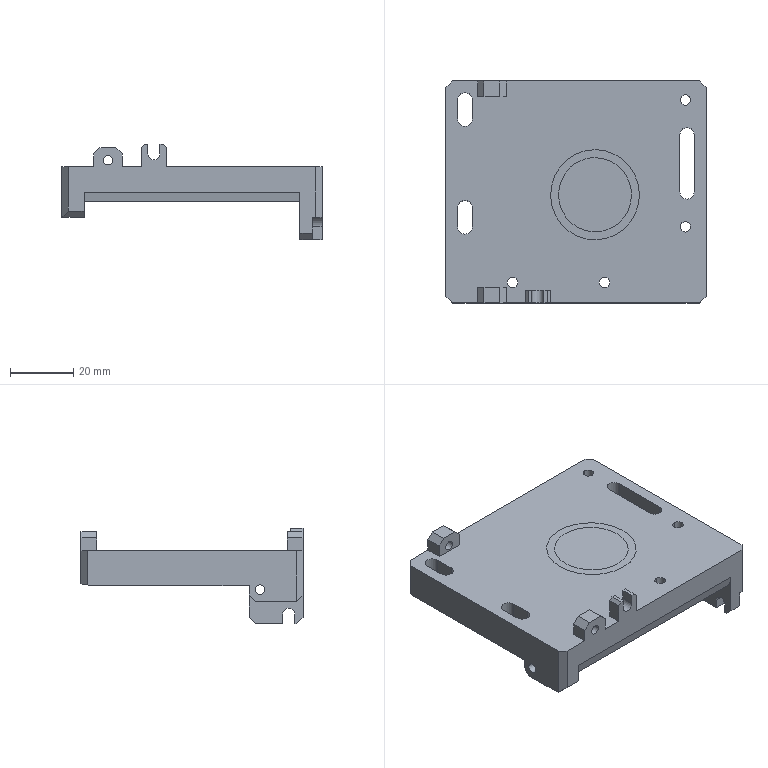NC program | NX | posted with a generic post | part box 82 x 70 x 30 mm
Lines 2139 to 2435 of 2435:
(FIXED_CONTOUR_COPY , TOOL : D3R0.5)
N4240 T05 M6
N4242 G54
N4244 G17 G0 G90 X-35.934 Y-39.23 B0. C0. S9500 M3
N4246 G43 Z30. H5
N4248 Z-9.
N4250 G94 G1 Z-12.53 F1000.
N4252 G2 X-36.039 Y-39.048 R0.21
N4254 G1 Y39.048 F2000.
N4256 X-35.992 Y39.095 Z-12.52
N4258 Y-39.095
N4260 X-35.945 Y-39.142 Z-12.512
N4262 Y39.142
N4264 X-35.897 Y39.189 Z-12.503
N4266 Y-39.189
N4268 X-35.85 Y-39.237 Z-12.495
N4270 Y39.237
N4272 X-35.803 Y39.284 Z-12.487
N4274 Y-39.284
N4276 X-35.756 Y-39.331 Z-12.478
N4278 Y39.331
N4280 X-35.709 Y39.378 Z-12.47
N4282 Y-39.378
N4284 X-35.662 Y-39.425 Z-12.462
N4286 Y39.425
N4288 X-35.614 Y39.472 Z-12.453
N4290 Y-39.472
N4292 X-35.567 Y-39.52 Z-12.445
N4294 Y39.52
N4296 X-35.52 Y39.567 Z-12.437
N4298 Y-39.567
N4300 X-35.473 Y-39.614 Z-12.428
N4302 Y39.614
N4304 X-35.426 Y39.661 Z-12.42
N4306 Y-39.661
N4308 X-35.378 Y-39.709 Z-12.412
N4310 Y39.709
N4312 X-35.331 Y39.756 Z-12.403
N4314 Y-39.756
N4316 X-35.284 Y-39.803 Z-12.395
N4318 Y39.803
N4320 X-35.236 Y39.851 Z-12.387
N4322 Y-39.851
N4324 X-35.189 Y-39.898 Z-12.378
N4326 Y39.898
N4328 X-35.142 Y39.945 Z-12.37
N4330 Y-39.945
N4332 X-35.094 Y-39.993 Z-12.362
N4334 Y39.993
N4336 X-35.047 Y40.04 Z-12.353
N4338 Y-40.04
N4340 X-35. Y-40.087 Z-12.345
N4342 Y40.087
N4344 X-34.952 Y40.135 Z-12.337
N4346 Y-40.135
N4348 X-34.905 Y-40.182 Z-12.328
N4350 Y40.182
N4352 X-34.857 Y40.23 Z-12.32
N4354 Y-40.23
N4356 X-34.81 Y-40.277 Z-12.311
N4358 Y40.277
N4360 X-34.763 Y40.324 Z-12.303
N4362 Y-40.324
N4364 X-34.715 Y-40.372 Z-12.295
N4366 Y40.372
N4368 X-34.668 Y40.419 Z-12.286
N4370 Y-40.419
N4372 X-34.62 Y-40.467 Z-12.278
N4374 Y40.467
N4376 X-34.573 Y40.514 Z-12.27
N4378 Y-40.514
N4380 X-34.526 Y-40.561 Z-12.261
N4382 Y40.561
N4384 X-34.478 Y40.609 Z-12.253
N4386 Y-40.609
N4388 X-34.431 Y-40.656 Z-12.245
N4390 Y40.656
N4392 X-34.383 Y40.703 Z-12.236
N4394 Y-40.703
N4396 X-34.336 Y-40.751 Z-12.228
N4398 Y40.751
N4400 X-34.289 Y40.798 Z-12.22
N4402 Y-40.798
N4404 X-34.242 Y-40.845 Z-12.211
N4406 X-34.241 Y40.845
N4408 X-34.194 Y40.893 Z-12.203
N4410 Y-40.893
N4412 X-34.147 Y-40.94 Z-12.195
N4414 Y40.94
N4416 X-34.099 Y40.988 Z-12.187
N4418 Y38.314 Z-12.186
N4420 Y-40.868
N4422 Y-40.988 Z-12.187
N4424 X-34.087 Y-41. Z-12.185
N4426 X-34.05 Z-12.179
N4428 Y-40.23 Z-12.177
N4430 Y40.868
N4432 Y41. Z-12.179
N4434 X-34.001 Z-12.17
N4436 Y40.23 Z-12.169
N4438 Y-40.868
N4440 Y-41. Z-12.17
N4442 X-33.951 Z-12.161
N4444 Y-40.23 Z-12.16
N4446 Y40.868
N4448 Y41. Z-12.161
N4450 X-33.902 Z-12.153
N4452 Y40.233 Z-12.151
N4454 Y-40.864
N4456 Y-41. Z-12.153
N4458 X-33.853 Z-12.144
N4460 Y-40.23 Z-12.143
N4462 Y40.868
N4464 Y41. Z-12.144
N4466 X-33.804 Z-12.135
N4468 Y40.23 Z-12.134
N4470 Y-40.868
N4472 Y-41. Z-12.135
N4474 X-33.754 Z-12.127
N4476 Y-40.23 Z-12.125
N4478 Y40.868
N4480 Y41. Z-12.127
N4482 X-33.705 Z-12.118
N4484 Y40.23 Z-12.117
N4486 Y-40.868
N4488 Y-41. Z-12.118
N4490 X-33.656 Z-12.109
N4492 Y-40.23 Z-12.108
N4494 Y40.868
N4496 Y41. Z-12.109
N4498 X-33.607 Z-12.101
N4500 Y40.23 Z-12.099
N4502 Y-40.868
N4504 Y-41. Z-12.101
N4506 X-33.557 Z-12.092
N4508 Y-40.23 Z-12.091
N4510 Y40.871
N4512 Y41. Z-12.092
N4514 X-33.508 Z-12.083
N4516 Y40.23 Z-12.082
N4518 Y-40.868
N4520 Y-41. Z-12.083
N4522 X-33.459 Z-12.075
N4524 Y-40.23 Z-12.073
N4526 Y40.868
N4528 Y41. Z-12.075
N4530 X-33.41 Z-12.066
N4532 Y40.23 Z-12.065
N4534 Y-40.868
N4536 Y-41. Z-12.066
N4538 X-33.36 Z-12.057
N4540 Y-40.23 Z-12.056
N4542 Y40.868
N4544 Y41. Z-12.057
N4546 X-33.311 Z-12.049
N4548 Y40.23 Z-12.047
N4550 Y-40.868
N4552 Y-41. Z-12.049
N4554 X-33.262 Z-12.04
N4556 Y-40.23 Z-12.038
N4558 Y40.868
N4560 Y41. Z-12.04
N4562 X-33.213 Z-12.031
N4564 Y40.233 Z-12.03
N4566 Y-40.868
N4568 Y-41. Z-12.031
N4570 X-33.163 Z-12.023
N4572 Y41.
N4574 X-33.114 Z-12.015
N4576 Y-41.
N4578 G2 X-33.264 Y-41.26 R0.3
N4580 G1 Z-9.
N4582 G0 Z30.
(ZLEVEL_PROFILE_1_COPY_COPY , TOOL : D3R0.5)
N4584 X36.666 Y32.722
N4586 Z-10.598
N4588 G1 Z-12.098 F1000.
N4590 X36.21 Y32.873
N4592 G3 X35.916 Y32.812 R0.3
N4594 G1 X35.908 Y32.805 F2500.
N4596 Y-32.805
N4598 X35.916 Y-32.812
N4600 X35.925 Y-32.819 Z-12.197
N4602 Y32.819
N4604 X35.943 Y32.833 Z-12.295
N4606 Y-32.833
N4608 X35.96 Y-32.848 Z-12.394
N4610 Y32.848
N4612 X35.977 Y32.862 Z-12.492
N4614 Y-32.862
N4616 X35.995 Y-32.877 Z-12.591
N4618 Y32.877
N4620 X36.012 Y32.893 Z-12.689
N4622 Y-32.893
N4624 X36.029 Y-32.909 Z-12.788
N4626 Y32.909
N4628 X36.047 Y32.926 Z-12.886
N4630 Y-32.926
N4632 X36.064 Y-32.943 Z-12.985
N4634 Y32.943
N4636 X36.082 Y32.961 Z-13.083
N4638 Y-32.961
N4640 X36.099 Y-32.979 Z-13.182
N4642 Y32.979
N4644 X36.116 Y32.998 Z-13.28
N4646 Y-32.998
N4648 X36.134 Y-33.018 Z-13.379
N4650 Y33.018
N4652 X36.151 Y33.038 Z-13.477
N4654 Y-33.038
N4656 X36.168 Y-33.059 Z-13.576
N4658 Y33.059
N4660 X36.186 Y33.081 Z-13.674
N4662 Y-33.081
N4664 X36.203 Y-33.104 Z-13.773
N4666 Y33.104
N4668 X36.221 Y33.128 Z-13.871
N4670 Y-33.128
N4672 X36.238 Y-33.153 Z-13.97
N4674 Y33.153
N4676 X36.255 Y33.179 Z-14.068
N4678 Y-33.179
N4680 X36.273 Y-33.206 Z-14.167
N4682 Y33.206
N4684 X36.29 Y33.234 Z-14.265
N4686 Y-33.234
N4688 X36.307 Y-33.265 Z-14.364
N4690 Y33.265
N4692 X36.325 Y33.296 Z-14.462
N4694 Y-33.296
N4696 X36.342 Y-33.33 Z-14.561
N4698 Y33.33
N4700 X36.359 Y33.366 Z-14.659
N4702 Y-33.366
N4704 X36.377 Y-33.405 Z-14.757
N4706 Y33.405
N4708 X36.394 Y33.447 Z-14.856
N4710 Y-33.447
N4712 X36.412 Y-33.492 Z-14.954
N4714 Y33.492
N4716 X36.429 Y33.544 Z-15.053
N4718 Y-33.544
N4720 X36.446 Y-33.602 Z-15.151
N4722 Y33.602
N4724 X36.462 Y33.663 Z-15.239
N4726 Y-33.663
N4728 X36.477 Y-33.738 Z-15.326
N4730 Y33.738
N4732 X36.492 Y33.54 Z-15.413
N4734 Y-33.54
N4736 X36.494 Y-33.662 Z-15.423
N4738 X36.496 Y-33.785 Z-15.432
N4740 X36.497 Y-33.907 Z-15.442
N4742 X36.5 Y-34.03 Z-15.452
N4744 X36.501 Y-34.152 Z-15.461
N4746 X36.503 Y-34.275 Z-15.471
N4748 X36.504 Y-34.397 Z-15.481
N4750 X36.505 Y-34.519 Z-15.49
N4752 X36.5 Y-34.642 Z-15.5
N4754 X36.508 Y-34.397
N4756 Y34.397
N4758 X36.5 Y34.642
N4760 G2 X36.642 Y34.906 R0.3
N4762 G1 X37.1 Y35.19
N4764 Z-14.
N4766 G0 Z30.
N4768 M5
(DRILLING , TOOL : D6A45)
N4770 T07 M6
N4772 G54
N4774 G17 G0 G90 X-29. Y-34.5 B0. C0. S5000 M3
N4776 G43 Z30. H7
N4778 G94 G81 G98 Z-14.025 F250. R-9.
N4780 X11.
N4782 X28.5 Y-9.
N4784 Y20.
N4786 G80
N4788 G0 X28.5 Y20. Z30.
(DRILLING_COPY , TOOL : 3.3ZT)
N4790 T13 M6
N4792 G17 G43 G0 G90 X-29. Y-34.5 Z30. B0. C0. S2000 H13 M3
N4794 G94 G83 G98 Z-25.491 F150. Q2. R-9.
N4796 X11.
N4798 X28.5 Y-9.
N4800 Y20.
N4802 G80
N4804 G0 X28.5 Y20. Z30.
N4806 M5
N4808 M2